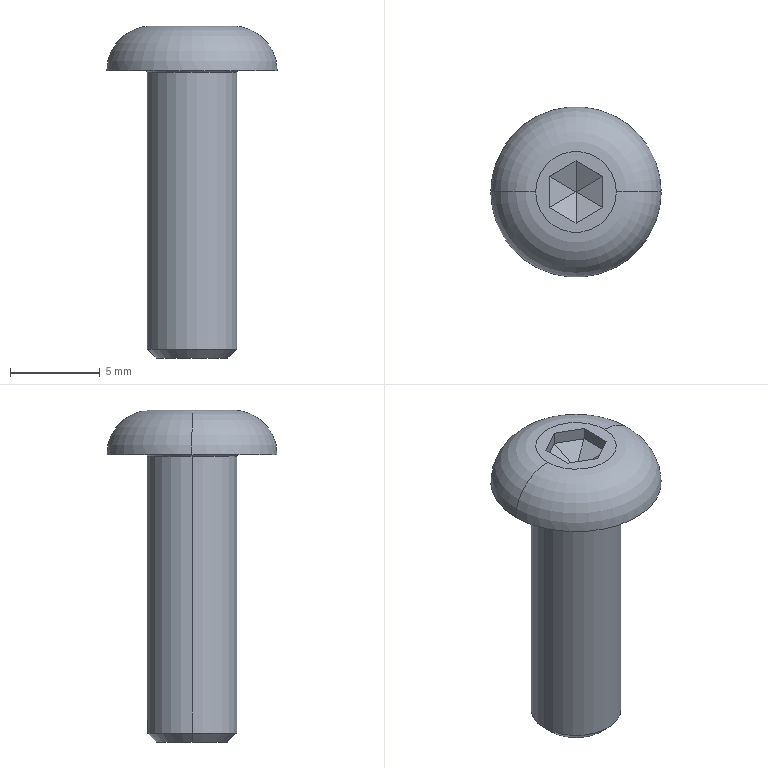Part | SolidWorks | features Chamfer 2, Fillet 2, ICE 2, Extrusion 1, RefAxis 1 | 1 solid | 24 faces | box 9.5 x 9.5 x 18.5 mm | volume 446.572 mm3 | plane 16 | torus 4 | cone 2 | cylinder 2 | commonest cylinder face diameters 5 x2
STEP:
#1=CARTESIAN_POINT('',(-2.6,0.,0.));
#2=VERTEX_POINT('',#1);
#3=CARTESIAN_POINT('',(2.6,0.,0.));
#4=VERTEX_POINT('',#3);
#5=CARTESIAN_POINT('',(0.,0.,0.));
#6=DIRECTION('',(0.,0.,1.));
#7=DIRECTION('',(1.,0.,0.));
#8=AXIS2_PLACEMENT_3D('',#5,#6,#7);
#9=CIRCLE('',#8,2.6);
#10=EDGE_CURVE('',#2,#4,#9,.T.);
#11=ORIENTED_EDGE('',*,*,#10,.F.);
#12=CARTESIAN_POINT('',(-2.5,0.,-0.1));
#13=VERTEX_POINT('',#12);
#14=CARTESIAN_POINT('',(-2.6,0.,-0.1));
#15=DIRECTION('',(0.,1.,0.));
#16=DIRECTION('',(-1.,0.,0.));
#17=AXIS2_PLACEMENT_3D('',#14,#15,#16);
#18=CIRCLE('',#17,0.1);
#19=EDGE_CURVE('',#2,#13,#18,.T.);
#20=ORIENTED_EDGE('',*,*,#19,.T.);
#21=CARTESIAN_POINT('',(2.5,0.,-0.1));
#22=VERTEX_POINT('',#21);
#23=CARTESIAN_POINT('',(0.,0.,-0.1));
#24=DIRECTION('',(0.,0.,-1.));
#25=DIRECTION('',(1.,0.,0.));
#26=AXIS2_PLACEMENT_3D('',#23,#24,#25);
#27=CIRCLE('',#26,2.5);
#28=EDGE_CURVE('',#22,#13,#27,.T.);
#29=ORIENTED_EDGE('',*,*,#28,.F.);
#30=CARTESIAN_POINT('',(2.6,0.,-0.1));
#31=DIRECTION('',(0.,-1.,0.));
#32=DIRECTION('',(0.,0.,-1.));
#33=AXIS2_PLACEMENT_3D('',#30,#31,#32);
#34=CIRCLE('',#33,0.1);
#35=EDGE_CURVE('',#4,#22,#34,.T.);
#36=ORIENTED_EDGE('',*,*,#35,.F.);
#37=EDGE_LOOP('',(#11,#20,#29,#36));
#38=FACE_OUTER_BOUND('',#37,.T.);
#39=CARTESIAN_POINT('',(0.,0.,-0.1));
#40=DIRECTION('',(0.,0.,1.));
#41=DIRECTION('',(1.,0.,0.));
#42=AXIS2_PLACEMENT_3D('',#39,#40,#41);
#43=TOROIDAL_SURFACE('',#42,2.6,0.1);
#44=ADVANCED_FACE('',(#38),#43,.F.);
#45=CARTESIAN_POINT('',(-2.,0.,-16.));
#46=VERTEX_POINT('',#45);
#47=CARTESIAN_POINT('',(2.,0.,-16.));
#48=VERTEX_POINT('',#47);
#49=CARTESIAN_POINT('',(0.,0.,-16.));
#50=DIRECTION('',(0.,0.,-1.));
#51=DIRECTION('',(-1.,0.,0.));
#52=AXIS2_PLACEMENT_3D('',#49,#50,#51);
#53=CIRCLE('',#52,2.);
#54=EDGE_CURVE('',#46,#48,#53,.T.);
#55=ORIENTED_EDGE('',*,*,#54,.F.);
#56=CARTESIAN_POINT('',(-2.5,0.,-15.5));
#57=VERTEX_POINT('',#56);
#58=CARTESIAN_POINT('',(-2.,0.,-16.));
#59=DIRECTION('',(-0.7071,0.,0.7071));
#60=VECTOR('',#59,1000.);
#61=LINE('',#58,#60);
#62=EDGE_CURVE('',#46,#57,#61,.T.);
#63=ORIENTED_EDGE('',*,*,#62,.T.);
#64=CARTESIAN_POINT('',(2.5,0.,-15.5));
#65=VERTEX_POINT('',#64);
#66=CARTESIAN_POINT('',(0.,0.,-15.5));
#67=DIRECTION('',(0.,0.,1.));
#68=DIRECTION('',(-1.,0.,0.));
#69=AXIS2_PLACEMENT_3D('',#66,#67,#68);
#70=CIRCLE('',#69,2.5);
#71=EDGE_CURVE('',#65,#57,#70,.T.);
#72=ORIENTED_EDGE('',*,*,#71,.F.);
#73=CARTESIAN_POINT('',(2.,0.,-16.));
#74=DIRECTION('',(0.7071,0.,0.7071));
#75=VECTOR('',#74,1000.);
#76=LINE('',#73,#75);
#77=EDGE_CURVE('',#48,#65,#76,.T.);
#78=ORIENTED_EDGE('',*,*,#77,.F.);
#79=EDGE_LOOP('',(#55,#63,#72,#78));
#80=FACE_OUTER_BOUND('',#79,.T.);
#81=CARTESIAN_POINT('',(0.,0.,-16.));
#82=DIRECTION('',(0.,0.,1.));
#83=DIRECTION('',(1.,0.,0.));
#84=AXIS2_PLACEMENT_3D('',#81,#82,#83);
#85=CONICAL_SURFACE('',#84,2.,0.7854);
#86=ADVANCED_FACE('',(#80),#85,.T.);
#87=ORIENTED_EDGE('',*,*,#71,.T.);
#88=CARTESIAN_POINT('',(-2.5,0.,-16.));
#89=DIRECTION('',(0.,0.,1.));
#90=VECTOR('',#89,1000.);
#91=LINE('',#88,#90);
#92=EDGE_CURVE('',#57,#13,#91,.T.);
#93=ORIENTED_EDGE('',*,*,#92,.T.);
#94=CARTESIAN_POINT('',(0.,0.,-0.1));
#95=DIRECTION('',(0.,0.,-1.));
#96=DIRECTION('',(1.,0.,0.));
#97=AXIS2_PLACEMENT_3D('',#94,#95,#96);
#98=CIRCLE('',#97,2.5);
#99=EDGE_CURVE('',#13,#22,#98,.T.);
#100=ORIENTED_EDGE('',*,*,#99,.T.);
#101=CARTESIAN_POINT('',(2.5,0.,-16.));
#102=DIRECTION('',(0.,0.,1.));
#103=VECTOR('',#102,1000.);
#104=LINE('',#101,#103);
#105=EDGE_CURVE('',#65,#22,#104,.T.);
#106=ORIENTED_EDGE('',*,*,#105,.F.);
#107=EDGE_LOOP('',(#87,#93,#100,#106));
#108=FACE_OUTER_BOUND('',#107,.T.);
#109=CARTESIAN_POINT('',(0.,0.,-16.));
#110=DIRECTION('',(0.,0.,1.));
#111=DIRECTION('',(1.,0.,0.));
#112=AXIS2_PLACEMENT_3D('',#109,#110,#111);
#113=CYLINDRICAL_SURFACE('',#112,2.5);
#114=ADVANCED_FACE('',(#108),#113,.T.);
#115=CARTESIAN_POINT('',(4.75,0.,0.));
#116=VERTEX_POINT('',#115);
#117=CARTESIAN_POINT('',(-4.75,0.,0.));
#118=VERTEX_POINT('',#117);
#119=CARTESIAN_POINT('',(0.,0.,0.));
#120=DIRECTION('',(0.,0.,1.));
#121=DIRECTION('',(1.,0.,0.));
#122=AXIS2_PLACEMENT_3D('',#119,#120,#121);
#123=CIRCLE('',#122,4.75);
#124=EDGE_CURVE('',#116,#118,#123,.T.);
#125=ORIENTED_EDGE('',*,*,#124,.T.);
#126=CARTESIAN_POINT('',(-2.25,0.,2.5));
#127=VERTEX_POINT('',#126);
#128=CARTESIAN_POINT('',(-2.25,0.,0.));
#129=DIRECTION('',(0.,1.,0.));
#130=DIRECTION('',(-1.,0.,0.));
#131=AXIS2_PLACEMENT_3D('',#128,#129,#130);
#132=CIRCLE('',#131,2.5);
#133=EDGE_CURVE('',#118,#127,#132,.T.);
#134=ORIENTED_EDGE('',*,*,#133,.T.);
#135=CARTESIAN_POINT('',(2.25,0.,2.5));
#136=VERTEX_POINT('',#135);
#137=CARTESIAN_POINT('',(0.,0.,2.5));
#138=DIRECTION('',(0.,0.,1.));
#139=DIRECTION('',(1.,0.,0.));
#140=AXIS2_PLACEMENT_3D('',#137,#138,#139);
#141=CIRCLE('',#140,2.25);
#142=EDGE_CURVE('',#136,#127,#141,.T.);
#143=ORIENTED_EDGE('',*,*,#142,.F.);
#144=CARTESIAN_POINT('',(2.25,0.,0.));
#145=DIRECTION('',(0.,-1.,0.));
#146=DIRECTION('',(0.,0.,-1.));
#147=AXIS2_PLACEMENT_3D('',#144,#145,#146);
#148=CIRCLE('',#147,2.5);
#149=EDGE_CURVE('',#116,#136,#148,.T.);
#150=ORIENTED_EDGE('',*,*,#149,.F.);
#151=EDGE_LOOP('',(#125,#134,#143,#150));
#152=FACE_OUTER_BOUND('',#151,.T.);
#153=CARTESIAN_POINT('',(0.,0.,0.));
#154=DIRECTION('',(0.,0.,1.));
#155=DIRECTION('',(1.,0.,0.));
#156=AXIS2_PLACEMENT_3D('',#153,#154,#155);
#157=TOROIDAL_SURFACE('',#156,2.25,2.5);
#158=ADVANCED_FACE('',(#152),#157,.T.);
#159=CARTESIAN_POINT('',(0.,0.,0.));
#160=DIRECTION('',(0.,0.,1.));
#161=DIRECTION('',(1.,0.,0.));
#162=AXIS2_PLACEMENT_3D('',#159,#160,#161);
#163=CIRCLE('',#162,2.6);
#164=EDGE_CURVE('',#4,#2,#163,.T.);
#165=ORIENTED_EDGE('',*,*,#164,.T.);
#166=ORIENTED_EDGE('',*,*,#10,.T.);
#167=EDGE_LOOP('',(#165,#166));
#168=FACE_BOUND('',#167,.T.);
#169=ORIENTED_EDGE('',*,*,#124,.F.);
#170=CARTESIAN_POINT('',(0.,0.,0.));
#171=DIRECTION('',(0.,0.,1.));
#172=DIRECTION('',(1.,0.,0.));
#173=AXIS2_PLACEMENT_3D('',#170,#171,#172);
#174=CIRCLE('',#173,4.75);
#175=EDGE_CURVE('',#118,#116,#174,.T.);
#176=ORIENTED_EDGE('',*,*,#175,.F.);
#177=EDGE_LOOP('',(#169,#176));
#178=FACE_OUTER_BOUND('',#177,.T.);
#179=CARTESIAN_POINT('',(0.,0.,0.));
#180=DIRECTION('',(0.,0.,1.));
#181=DIRECTION('',(1.,0.,0.));
#182=AXIS2_PLACEMENT_3D('',#179,#180,#181);
#183=PLANE('',#182);
#184=ADVANCED_FACE('',(#168,#178),#183,.F.);
#185=CARTESIAN_POINT('',(1.5,-0.866,2.5));
#186=VERTEX_POINT('',#185);
#187=CARTESIAN_POINT('',(1.5,0.866,2.5));
#188=VERTEX_POINT('',#187);
#189=CARTESIAN_POINT('',(1.5,-0.866,2.5));
#190=DIRECTION('',(0.,1.,0.));
#191=VECTOR('',#190,1000.);
#192=LINE('',#189,#191);
#193=EDGE_CURVE('',#186,#188,#192,.T.);
#194=ORIENTED_EDGE('',*,*,#193,.F.);
#195=CARTESIAN_POINT('',(0.,-1.732,2.5));
#196=VERTEX_POINT('',#195);
#197=CARTESIAN_POINT('',(0.,-1.732,2.5));
#198=DIRECTION('',(0.866,0.5,0.));
#199=VECTOR('',#198,1000.);
#200=LINE('',#197,#199);
#201=EDGE_CURVE('',#196,#186,#200,.T.);
#202=ORIENTED_EDGE('',*,*,#201,.F.);
#203=CARTESIAN_POINT('',(-1.5,-0.866,2.5));
#204=VERTEX_POINT('',#203);
#205=CARTESIAN_POINT('',(-1.5,-0.866,2.5));
#206=DIRECTION('',(0.866,-0.5,0.));
#207=VECTOR('',#206,1000.);
#208=LINE('',#205,#207);
#209=EDGE_CURVE('',#204,#196,#208,.T.);
#210=ORIENTED_EDGE('',*,*,#209,.F.);
#211=CARTESIAN_POINT('',(-1.5,0.866,2.5));
#212=VERTEX_POINT('',#211);
#213=CARTESIAN_POINT('',(-1.5,0.866,2.5));
#214=DIRECTION('',(0.,-1.,0.));
#215=VECTOR('',#214,1000.);
#216=LINE('',#213,#215);
#217=EDGE_CURVE('',#212,#204,#216,.T.);
#218=ORIENTED_EDGE('',*,*,#217,.F.);
#219=CARTESIAN_POINT('',(0.,1.732,2.5));
#220=VERTEX_POINT('',#219);
#221=CARTESIAN_POINT('',(0.,1.732,2.5));
#222=DIRECTION('',(-0.866,-0.5,0.));
#223=VECTOR('',#222,1000.);
#224=LINE('',#221,#223);
#225=EDGE_CURVE('',#220,#212,#224,.T.);
#226=ORIENTED_EDGE('',*,*,#225,.F.);
#227=CARTESIAN_POINT('',(1.5,0.866,2.5));
#228=DIRECTION('',(-0.866,0.5,0.));
#229=VECTOR('',#228,1000.);
#230=LINE('',#227,#229);
#231=EDGE_CURVE('',#188,#220,#230,.T.);
#232=ORIENTED_EDGE('',*,*,#231,.F.);
#233=EDGE_LOOP('',(#194,#202,#210,#218,#226,#232));
#234=FACE_BOUND('',#233,.T.);
#235=ORIENTED_EDGE('',*,*,#142,.T.);
#236=CARTESIAN_POINT('',(0.,0.,2.5));
#237=DIRECTION('',(0.,0.,1.));
#238=DIRECTION('',(1.,0.,0.));
#239=AXIS2_PLACEMENT_3D('',#236,#237,#238);
#240=CIRCLE('',#239,2.25);
#241=EDGE_CURVE('',#127,#136,#240,.T.);
#242=ORIENTED_EDGE('',*,*,#241,.T.);
#243=EDGE_LOOP('',(#235,#242));
#244=FACE_OUTER_BOUND('',#243,.T.);
#245=CARTESIAN_POINT('',(0.,0.,2.5));
#246=DIRECTION('',(0.,0.,1.));
#247=DIRECTION('',(1.,0.,0.));
#248=AXIS2_PLACEMENT_3D('',#245,#246,#247);
#249=PLANE('',#248);
#250=ADVANCED_FACE('',(#234,#244),#249,.T.);
#251=ORIENTED_EDGE('',*,*,#133,.F.);
#252=ORIENTED_EDGE('',*,*,#175,.T.);
#253=ORIENTED_EDGE('',*,*,#149,.T.);
#254=ORIENTED_EDGE('',*,*,#241,.F.);
#255=EDGE_LOOP('',(#251,#252,#253,#254));
#256=FACE_OUTER_BOUND('',#255,.T.);
#257=CARTESIAN_POINT('',(0.,0.,0.));
#258=DIRECTION('',(0.,0.,1.));
#259=DIRECTION('',(1.,0.,0.));
#260=AXIS2_PLACEMENT_3D('',#257,#258,#259);
#261=TOROIDAL_SURFACE('',#260,2.25,2.5);
#262=ADVANCED_FACE('',(#256),#261,.T.);
#263=ORIENTED_EDGE('',*,*,#92,.F.);
#264=CARTESIAN_POINT('',(0.,0.,-15.5));
#265=DIRECTION('',(0.,0.,1.));
#266=DIRECTION('',(-1.,0.,0.));
#267=AXIS2_PLACEMENT_3D('',#264,#265,#266);
#268=CIRCLE('',#267,2.5);
#269=EDGE_CURVE('',#57,#65,#268,.T.);
#270=ORIENTED_EDGE('',*,*,#269,.T.);
#271=ORIENTED_EDGE('',*,*,#105,.T.);
#272=ORIENTED_EDGE('',*,*,#28,.T.);
#273=EDGE_LOOP('',(#263,#270,#271,#272));
#274=FACE_OUTER_BOUND('',#273,.T.);
#275=CARTESIAN_POINT('',(0.,0.,-16.));
#276=DIRECTION('',(0.,0.,1.));
#277=DIRECTION('',(1.,0.,0.));
#278=AXIS2_PLACEMENT_3D('',#275,#276,#277);
#279=CYLINDRICAL_SURFACE('',#278,2.5);
#280=ADVANCED_FACE('',(#274),#279,.T.);
#281=CARTESIAN_POINT('',(0.,0.,-16.));
#282=DIRECTION('',(0.,0.,-1.));
#283=DIRECTION('',(-1.,0.,0.));
#284=AXIS2_PLACEMENT_3D('',#281,#282,#283);
#285=CIRCLE('',#284,2.);
#286=EDGE_CURVE('',#48,#46,#285,.T.);
#287=ORIENTED_EDGE('',*,*,#286,.T.);
#288=ORIENTED_EDGE('',*,*,#54,.T.);
#289=EDGE_LOOP('',(#287,#288));
#290=FACE_OUTER_BOUND('',#289,.T.);
#291=CARTESIAN_POINT('',(0.,0.,-16.));
#292=DIRECTION('',(0.,0.,-1.));
#293=DIRECTION('',(-1.,0.,0.));
#294=AXIS2_PLACEMENT_3D('',#291,#292,#293);
#295=PLANE('',#294);
#296=ADVANCED_FACE('',(#290),#295,.T.);
#297=CARTESIAN_POINT('',(1.5,0.866,1.805));
#298=VERTEX_POINT('',#297);
#299=CARTESIAN_POINT('',(1.5,0.866,0.94));
#300=DIRECTION('',(0.,0.,1.));
#301=VECTOR('',#300,1000.);
#302=LINE('',#299,#301);
#303=EDGE_CURVE('',#298,#188,#302,.T.);
#304=ORIENTED_EDGE('',*,*,#303,.F.);
#305=CARTESIAN_POINT('',(1.5,-0.866,1.805));
#306=VERTEX_POINT('',#305);
#307=CARTESIAN_POINT('',(1.5,-0.866,1.805));
#308=DIRECTION('',(0.,-1.,0.));
#309=VECTOR('',#308,1000.);
#310=LINE('',#307,#309);
#311=EDGE_CURVE('',#298,#306,#310,.T.);
#312=ORIENTED_EDGE('',*,*,#311,.T.);
#313=CARTESIAN_POINT('',(1.5,-0.866,0.94));
#314=DIRECTION('',(0.,0.,1.));
#315=VECTOR('',#314,1000.);
#316=LINE('',#313,#315);
#317=EDGE_CURVE('',#306,#186,#316,.T.);
#318=ORIENTED_EDGE('',*,*,#317,.T.);
#319=ORIENTED_EDGE('',*,*,#193,.T.);
#320=EDGE_LOOP('',(#304,#312,#318,#319));
#321=FACE_OUTER_BOUND('',#320,.T.);
#322=CARTESIAN_POINT('',(1.5,-0.866,0.94));
#323=DIRECTION('',(1.,0.,0.));
#324=DIRECTION('',(0.,1.,0.));
#325=AXIS2_PLACEMENT_3D('',#322,#323,#324);
#326=PLANE('',#325);
#327=ADVANCED_FACE('',(#321),#326,.F.);
#328=ORIENTED_EDGE('',*,*,#317,.F.);
#329=CARTESIAN_POINT('',(0.,-1.732,1.805));
#330=VERTEX_POINT('',#329);
#331=CARTESIAN_POINT('',(0.,-1.732,1.805));
#332=DIRECTION('',(-0.866,-0.5,0.));
#333=VECTOR('',#332,1000.);
#334=LINE('',#331,#333);
#335=EDGE_CURVE('',#306,#330,#334,.T.);
#336=ORIENTED_EDGE('',*,*,#335,.T.);
#337=CARTESIAN_POINT('',(0.,-1.732,0.94));
#338=DIRECTION('',(0.,0.,1.));
#339=VECTOR('',#338,1000.);
#340=LINE('',#337,#339);
#341=EDGE_CURVE('',#330,#196,#340,.T.);
#342=ORIENTED_EDGE('',*,*,#341,.T.);
#343=ORIENTED_EDGE('',*,*,#201,.T.);
#344=EDGE_LOOP('',(#328,#336,#342,#343));
#345=FACE_OUTER_BOUND('',#344,.T.);
#346=CARTESIAN_POINT('',(0.,-1.732,0.94));
#347=DIRECTION('',(0.5,-0.866,0.));
#348=DIRECTION('',(0.866,0.5,0.));
#349=AXIS2_PLACEMENT_3D('',#346,#347,#348);
#350=PLANE('',#349);
#351=ADVANCED_FACE('',(#345),#350,.F.);
#352=ORIENTED_EDGE('',*,*,#341,.F.);
#353=CARTESIAN_POINT('',(-1.5,-0.866,1.805));
#354=VERTEX_POINT('',#353);
#355=CARTESIAN_POINT('',(-1.5,-0.866,1.805));
#356=DIRECTION('',(-0.866,0.5,0.));
#357=VECTOR('',#356,1000.);
#358=LINE('',#355,#357);
#359=EDGE_CURVE('',#330,#354,#358,.T.);
#360=ORIENTED_EDGE('',*,*,#359,.T.);
#361=CARTESIAN_POINT('',(-1.5,-0.866,0.94));
#362=DIRECTION('',(0.,0.,1.));
#363=VECTOR('',#362,1000.);
#364=LINE('',#361,#363);
#365=EDGE_CURVE('',#354,#204,#364,.T.);
#366=ORIENTED_EDGE('',*,*,#365,.T.);
#367=ORIENTED_EDGE('',*,*,#209,.T.);
#368=EDGE_LOOP('',(#352,#360,#366,#367));
#369=FACE_OUTER_BOUND('',#368,.T.);
#370=CARTESIAN_POINT('',(-1.5,-0.866,0.94));
#371=DIRECTION('',(-0.5,-0.866,0.));
#372=DIRECTION('',(0.866,-0.5,0.));
#373=AXIS2_PLACEMENT_3D('',#370,#371,#372);
#374=PLANE('',#373);
#375=ADVANCED_FACE('',(#369),#374,.F.);
#376=ORIENTED_EDGE('',*,*,#365,.F.);
#377=CARTESIAN_POINT('',(-1.5,0.866,1.805));
#378=VERTEX_POINT('',#377);
#379=CARTESIAN_POINT('',(-1.5,0.866,1.805));
#380=DIRECTION('',(0.,1.,0.));
#381=VECTOR('',#380,1000.);
#382=LINE('',#379,#381);
#383=EDGE_CURVE('',#354,#378,#382,.T.);
#384=ORIENTED_EDGE('',*,*,#383,.T.);
#385=CARTESIAN_POINT('',(-1.5,0.866,0.94));
#386=DIRECTION('',(0.,0.,1.));
#387=VECTOR('',#386,1000.);
#388=LINE('',#385,#387);
#389=EDGE_CURVE('',#378,#212,#388,.T.);
#390=ORIENTED_EDGE('',*,*,#389,.T.);
#391=ORIENTED_EDGE('',*,*,#217,.T.);
#392=EDGE_LOOP('',(#376,#384,#390,#391));
#393=FACE_OUTER_BOUND('',#392,.T.);
#394=CARTESIAN_POINT('',(-1.5,0.866,0.94));
#395=DIRECTION('',(-1.,0.,0.));
#396=DIRECTION('',(0.,-1.,0.));
#397=AXIS2_PLACEMENT_3D('',#394,#395,#396);
#398=PLANE('',#397);
#399=ADVANCED_FACE('',(#393),#398,.F.);
#400=ORIENTED_EDGE('',*,*,#389,.F.);
#401=CARTESIAN_POINT('',(0.,1.732,1.805));
#402=VERTEX_POINT('',#401);
#403=CARTESIAN_POINT('',(0.,1.732,1.805));
#404=DIRECTION('',(0.866,0.5,0.));
#405=VECTOR('',#404,1000.);
#406=LINE('',#403,#405);
#407=EDGE_CURVE('',#378,#402,#406,.T.);
#408=ORIENTED_EDGE('',*,*,#407,.T.);
#409=CARTESIAN_POINT('',(0.,1.732,0.94));
#410=DIRECTION('',(0.,0.,1.));
#411=VECTOR('',#410,1000.);
#412=LINE('',#409,#411);
#413=EDGE_CURVE('',#402,#220,#412,.T.);
#414=ORIENTED_EDGE('',*,*,#413,.T.);
#415=ORIENTED_EDGE('',*,*,#225,.T.);
#416=EDGE_LOOP('',(#400,#408,#414,#415));
#417=FACE_OUTER_BOUND('',#416,.T.);
#418=CARTESIAN_POINT('',(0.,1.732,0.94));
#419=DIRECTION('',(-0.5,0.866,0.));
#420=DIRECTION('',(-0.866,-0.5,0.));
#421=AXIS2_PLACEMENT_3D('',#418,#419,#420);
#422=PLANE('',#421);
#423=ADVANCED_FACE('',(#417),#422,.F.);
#424=ORIENTED_EDGE('',*,*,#413,.F.);
#425=CARTESIAN_POINT('',(1.5,0.866,1.805));
#426=DIRECTION('',(0.866,-0.5,0.));
#427=VECTOR('',#426,1000.);
#428=LINE('',#425,#427);
#429=EDGE_CURVE('',#402,#298,#428,.T.);
#430=ORIENTED_EDGE('',*,*,#429,.T.);
#431=ORIENTED_EDGE('',*,*,#303,.T.);
#432=ORIENTED_EDGE('',*,*,#231,.T.);
#433=EDGE_LOOP('',(#424,#430,#431,#432));
#434=FACE_OUTER_BOUND('',#433,.T.);
#435=CARTESIAN_POINT('',(1.5,0.866,0.94));
#436=DIRECTION('',(0.5,0.866,0.));
#437=DIRECTION('',(-0.866,0.5,0.));
#438=AXIS2_PLACEMENT_3D('',#435,#436,#437);
#439=PLANE('',#438);
#440=ADVANCED_FACE('',(#434),#439,.F.);
#441=CARTESIAN_POINT('',(-0.00255,0.001472,0.94));
#442=VERTEX_POINT('',#441);
#443=CARTESIAN_POINT('',(-0.00255,-0.001472,0.94));
#444=VERTEX_POINT('',#443);
#445=CARTESIAN_POINT('',(-0.00255,0.,0.94));
#446=DIRECTION('',(0.,-1.,0.));
#447=VECTOR('',#446,1000.);
#448=LINE('',#445,#447);
#449=EDGE_CURVE('',#442,#444,#448,.T.);
#450=ORIENTED_EDGE('',*,*,#449,.T.);
#451=CARTESIAN_POINT('',(0.,-0.002944,0.94));
#452=VERTEX_POINT('',#451);
#453=CARTESIAN_POINT('',(-0.001275,-0.002208,0.94));
#454=DIRECTION('',(0.866,-0.5,0.));
#455=VECTOR('',#454,1000.);
#456=LINE('',#453,#455);
#457=EDGE_CURVE('',#444,#452,#456,.T.);
#458=ORIENTED_EDGE('',*,*,#457,.T.);
#459=CARTESIAN_POINT('',(0.00255,-0.001472,0.94));
#460=VERTEX_POINT('',#459);
#461=CARTESIAN_POINT('',(0.001275,-0.002208,0.94));
#462=DIRECTION('',(0.866,0.5,0.));
#463=VECTOR('',#462,1000.);
#464=LINE('',#461,#463);
#465=EDGE_CURVE('',#452,#460,#464,.T.);
#466=ORIENTED_EDGE('',*,*,#465,.T.);
#467=CARTESIAN_POINT('',(0.00255,0.001472,0.94));
#468=VERTEX_POINT('',#467);
#469=CARTESIAN_POINT('',(0.00255,0.,0.94));
#470=DIRECTION('',(0.,1.,0.));
#471=VECTOR('',#470,1000.);
#472=LINE('',#469,#471);
#473=EDGE_CURVE('',#460,#468,#472,.T.);
#474=ORIENTED_EDGE('',*,*,#473,.T.);
#475=CARTESIAN_POINT('',(0.,0.002944,0.94));
#476=VERTEX_POINT('',#475);
#477=CARTESIAN_POINT('',(0.001275,0.002208,0.94));
#478=DIRECTION('',(-0.866,0.5,0.));
#479=VECTOR('',#478,1000.);
#480=LINE('',#477,#479);
#481=EDGE_CURVE('',#468,#476,#480,.T.);
#482=ORIENTED_EDGE('',*,*,#481,.T.);
#483=CARTESIAN_POINT('',(-0.001275,0.002208,0.94));
#484=DIRECTION('',(-0.866,-0.5,0.));
#485=VECTOR('',#484,1000.);
#486=LINE('',#483,#485);
#487=EDGE_CURVE('',#476,#442,#486,.T.);
#488=ORIENTED_EDGE('',*,*,#487,.T.);
#489=EDGE_LOOP('',(#450,#458,#466,#474,#482,#488));
#490=FACE_OUTER_BOUND('',#489,.T.);
#491=CARTESIAN_POINT('',(0.,0.,0.94));
#492=DIRECTION('',(0.,0.,1.));
#493=DIRECTION('',(1.,0.,0.));
#494=AXIS2_PLACEMENT_3D('',#491,#492,#493);
#495=PLANE('',#494);
#496=ADVANCED_FACE('',(#490),#495,.T.);
#497=ORIENTED_EDGE('',*,*,#62,.F.);
#498=ORIENTED_EDGE('',*,*,#286,.F.);
#499=ORIENTED_EDGE('',*,*,#77,.T.);
#500=ORIENTED_EDGE('',*,*,#269,.F.);
#501=EDGE_LOOP('',(#497,#498,#499,#500));
#502=FACE_OUTER_BOUND('',#501,.T.);
#503=CARTESIAN_POINT('',(0.,0.,-16.));
#504=DIRECTION('',(0.,0.,1.));
#505=DIRECTION('',(1.,0.,0.));
#506=AXIS2_PLACEMENT_3D('',#503,#504,#505);
#507=CONICAL_SURFACE('',#506,2.,0.7854);
#508=ADVANCED_FACE('',(#502),#507,.T.);
#509=CARTESIAN_POINT('',(0.00204,0.001178,0.9397));
#510=DIRECTION('',(-0.7746,-0.4472,-0.4472));
#511=VECTOR('',#510,1000.);
#512=LINE('',#509,#511);
#513=EDGE_CURVE('',#298,#468,#512,.T.);
#514=ORIENTED_EDGE('',*,*,#513,.F.);
#515=ORIENTED_EDGE('',*,*,#429,.F.);
#516=CARTESIAN_POINT('',(0.,0.002355,0.9397));
#517=DIRECTION('',(0.,0.8944,0.4472));
#518=VECTOR('',#517,1000.);
#519=LINE('',#516,#518);
#520=EDGE_CURVE('',#476,#402,#519,.T.);
#521=ORIENTED_EDGE('',*,*,#520,.F.);
#522=ORIENTED_EDGE('',*,*,#481,.F.);
#523=EDGE_LOOP('',(#514,#515,#521,#522));
#524=FACE_OUTER_BOUND('',#523,.T.);
#525=CARTESIAN_POINT('',(0.001275,0.002208,0.94));
#526=DIRECTION('',(0.25,0.433,-0.866));
#527=DIRECTION('',(-0.866,0.5,0.));
#528=AXIS2_PLACEMENT_3D('',#525,#526,#527);
#529=PLANE('',#528);
#530=ADVANCED_FACE('',(#524),#529,.F.);
#531=ORIENTED_EDGE('',*,*,#520,.T.);
#532=ORIENTED_EDGE('',*,*,#407,.F.);
#533=CARTESIAN_POINT('',(-0.00204,0.001178,0.9397));
#534=DIRECTION('',(-0.7746,0.4472,0.4472));
#535=VECTOR('',#534,1000.);
#536=LINE('',#533,#535);
#537=EDGE_CURVE('',#442,#378,#536,.T.);
#538=ORIENTED_EDGE('',*,*,#537,.F.);
#539=ORIENTED_EDGE('',*,*,#487,.F.);
#540=EDGE_LOOP('',(#531,#532,#538,#539));
#541=FACE_OUTER_BOUND('',#540,.T.);
#542=CARTESIAN_POINT('',(-0.001275,0.002208,0.94));
#543=DIRECTION('',(-0.25,0.433,-0.866));
#544=DIRECTION('',(-0.866,-0.5,0.));
#545=AXIS2_PLACEMENT_3D('',#542,#543,#544);
#546=PLANE('',#545);
#547=ADVANCED_FACE('',(#541),#546,.F.);
#548=ORIENTED_EDGE('',*,*,#513,.T.);
#549=ORIENTED_EDGE('',*,*,#473,.F.);
#550=CARTESIAN_POINT('',(0.00204,-0.001178,0.9397));
#551=DIRECTION('',(-0.7746,0.4472,-0.4472));
#552=VECTOR('',#551,1000.);
#553=LINE('',#550,#552);
#554=EDGE_CURVE('',#306,#460,#553,.T.);
#555=ORIENTED_EDGE('',*,*,#554,.F.);
#556=ORIENTED_EDGE('',*,*,#311,.F.);
#557=EDGE_LOOP('',(#548,#549,#555,#556));
#558=FACE_OUTER_BOUND('',#557,.T.);
#559=CARTESIAN_POINT('',(0.00255,0.,0.94));
#560=DIRECTION('',(0.5,0.,-0.866));
#561=DIRECTION('',(0.,1.,0.));
#562=AXIS2_PLACEMENT_3D('',#559,#560,#561);
#563=PLANE('',#562);
#564=ADVANCED_FACE('',(#558),#563,.F.);
#565=ORIENTED_EDGE('',*,*,#537,.T.);
#566=ORIENTED_EDGE('',*,*,#383,.F.);
#567=CARTESIAN_POINT('',(-0.00204,-0.001178,0.9397));
#568=DIRECTION('',(-0.7746,-0.4472,0.4472));
#569=VECTOR('',#568,1000.);
#570=LINE('',#567,#569);
#571=EDGE_CURVE('',#444,#354,#570,.T.);
#572=ORIENTED_EDGE('',*,*,#571,.F.);
#573=ORIENTED_EDGE('',*,*,#449,.F.);
#574=EDGE_LOOP('',(#565,#566,#572,#573));
#575=FACE_OUTER_BOUND('',#574,.T.);
#576=CARTESIAN_POINT('',(-0.00255,0.,0.94));
#577=DIRECTION('',(-0.5,0.,-0.866));
#578=DIRECTION('',(0.,-1.,0.));
#579=AXIS2_PLACEMENT_3D('',#576,#577,#578);
#580=PLANE('',#579);
#581=ADVANCED_FACE('',(#575),#580,.F.);
#582=ORIENTED_EDGE('',*,*,#554,.T.);
#583=ORIENTED_EDGE('',*,*,#465,.F.);
#584=CARTESIAN_POINT('',(0.,-0.002355,0.9397));
#585=DIRECTION('',(0.,0.8944,-0.4472));
#586=VECTOR('',#585,1000.);
#587=LINE('',#584,#586);
#588=EDGE_CURVE('',#330,#452,#587,.T.);
#589=ORIENTED_EDGE('',*,*,#588,.F.);
#590=ORIENTED_EDGE('',*,*,#335,.F.);
#591=EDGE_LOOP('',(#582,#583,#589,#590));
#592=FACE_OUTER_BOUND('',#591,.T.);
#593=CARTESIAN_POINT('',(0.001275,-0.002208,0.94));
#594=DIRECTION('',(0.25,-0.433,-0.866));
#595=DIRECTION('',(0.866,0.5,0.));
#596=AXIS2_PLACEMENT_3D('',#593,#594,#595);
#597=PLANE('',#596);
#598=ADVANCED_FACE('',(#592),#597,.F.);
#599=ORIENTED_EDGE('',*,*,#571,.T.);
#600=ORIENTED_EDGE('',*,*,#359,.F.);
#601=ORIENTED_EDGE('',*,*,#588,.T.);
#602=ORIENTED_EDGE('',*,*,#457,.F.);
#603=EDGE_LOOP('',(#599,#600,#601,#602));
#604=FACE_OUTER_BOUND('',#603,.T.);
#605=CARTESIAN_POINT('',(-0.001275,-0.002208,0.94));
#606=DIRECTION('',(-0.25,-0.433,-0.866));
#607=DIRECTION('',(0.866,-0.5,0.));
#608=AXIS2_PLACEMENT_3D('',#605,#606,#607);
#609=PLANE('',#608);
#610=ADVANCED_FACE('',(#604),#609,.F.);
#611=ORIENTED_EDGE('',*,*,#19,.F.);
#612=ORIENTED_EDGE('',*,*,#164,.F.);
#613=ORIENTED_EDGE('',*,*,#35,.T.);
#614=ORIENTED_EDGE('',*,*,#99,.F.);
#615=EDGE_LOOP('',(#611,#612,#613,#614));
#616=FACE_OUTER_BOUND('',#615,.T.);
#617=CARTESIAN_POINT('',(0.,0.,-0.1));
#618=DIRECTION('',(0.,0.,1.));
#619=DIRECTION('',(1.,0.,0.));
#620=AXIS2_PLACEMENT_3D('',#617,#618,#619);
#621=TOROIDAL_SURFACE('',#620,2.6,0.1);
#622=ADVANCED_FACE('',(#616),#621,.F.);
#623=CLOSED_SHELL('',(#44,#86,#114,#158,#184,#250,#262,#280,#296,#327,#351,#375,#399,#423,#440,#496,#508,#530,#547,#564,#581,#598,#610,#622));
#624=MANIFOLD_SOLID_BREP('',#623);
#625=CARTESIAN_POINT('',(0.,0.,0.));
#626=DIRECTION('',(0.,0.,1.));
#627=DIRECTION('',(1.,0.,0.));
#628=AXIS2_PLACEMENT_3D('',#625,#626,#627);
#629=(LENGTH_UNIT()NAMED_UNIT(*)SI_UNIT(.MILLI.,.METRE.));
#630=UNCERTAINTY_MEASURE_WITH_UNIT(LENGTH_MEASURE(0.00001),#629,'','');
#631=(NAMED_UNIT(*)PLANE_ANGLE_UNIT()SI_UNIT($,.RADIAN.));
#632=(NAMED_UNIT(*)SI_UNIT($,.STERADIAN.)SOLID_ANGLE_UNIT());
#633=(GEOMETRIC_REPRESENTATION_CONTEXT(3)GLOBAL_UNCERTAINTY_ASSIGNED_CONTEXT((#630))GLOBAL_UNIT_ASSIGNED_CONTEXT((#629,#631,#632))REPRESENTATION_CONTEXT('',''));
#634=ADVANCED_BREP_SHAPE_REPRESENTATION('',(#624,#628),#633);